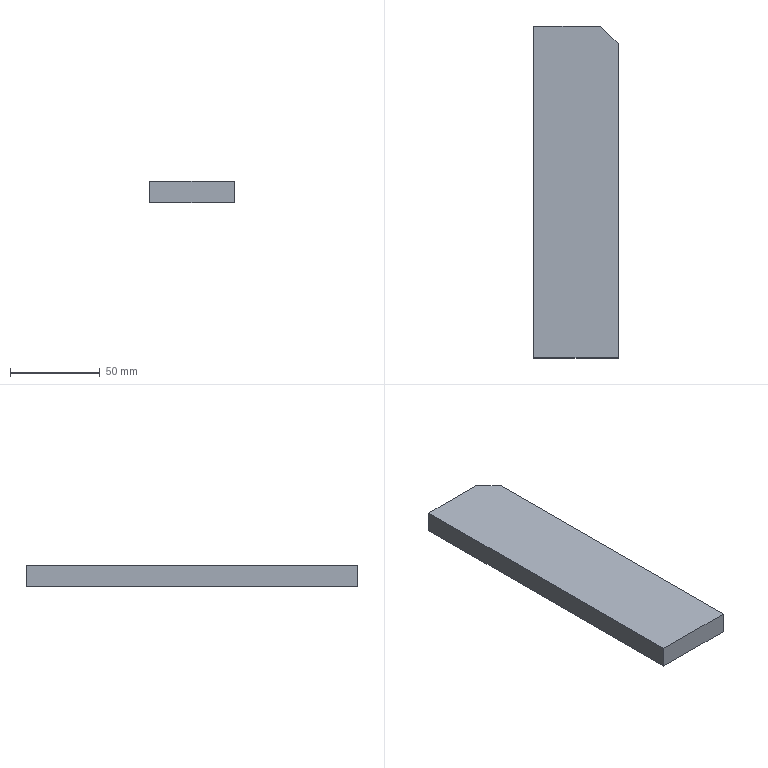Part | SolidWorks | features Chamfer 1, Extrusion 1, Fillet 1, ICE 1 | 1 solid | 7 faces | box 47 x 185 x 12 mm | volume 103740 mm3 | plane 7
STEP:
#1=CARTESIAN_POINT('',(0.,185.,-6.));
#2=VERTEX_POINT('',#1);
#3=CARTESIAN_POINT('',(0.,0.,-6.));
#4=VERTEX_POINT('',#3);
#5=CARTESIAN_POINT('',(0.,185.,-6.));
#6=DIRECTION('',(0.,-1.,0.));
#7=VECTOR('',#6,1000.);
#8=LINE('',#5,#7);
#9=EDGE_CURVE('',#2,#4,#8,.T.);
#10=ORIENTED_EDGE('',*,*,#9,.T.);
#11=CARTESIAN_POINT('',(0.,0.,6.));
#12=VERTEX_POINT('',#11);
#13=CARTESIAN_POINT('',(0.,0.,6.));
#14=DIRECTION('',(0.,0.,-1.));
#15=VECTOR('',#14,1000.);
#16=LINE('',#13,#15);
#17=EDGE_CURVE('',#12,#4,#16,.T.);
#18=ORIENTED_EDGE('',*,*,#17,.F.);
#19=CARTESIAN_POINT('',(0.,185.,6.));
#20=VERTEX_POINT('',#19);
#21=CARTESIAN_POINT('',(0.,185.,6.));
#22=DIRECTION('',(0.,-1.,0.));
#23=VECTOR('',#22,1000.);
#24=LINE('',#21,#23);
#25=EDGE_CURVE('',#20,#12,#24,.T.);
#26=ORIENTED_EDGE('',*,*,#25,.F.);
#27=CARTESIAN_POINT('',(0.,185.,6.));
#28=DIRECTION('',(0.,0.,-1.));
#29=VECTOR('',#28,1000.);
#30=LINE('',#27,#29);
#31=EDGE_CURVE('',#20,#2,#30,.T.);
#32=ORIENTED_EDGE('',*,*,#31,.T.);
#33=EDGE_LOOP('',(#10,#18,#26,#32));
#34=FACE_OUTER_BOUND('',#33,.T.);
#35=CARTESIAN_POINT('',(0.,185.,6.));
#36=DIRECTION('',(1.,0.,0.));
#37=DIRECTION('',(0.,0.,-1.));
#38=AXIS2_PLACEMENT_3D('',#35,#36,#37);
#39=PLANE('',#38);
#40=ADVANCED_FACE('',(#34),#39,.F.);
#41=CARTESIAN_POINT('',(47.,0.,-6.));
#42=VERTEX_POINT('',#41);
#43=CARTESIAN_POINT('',(0.,0.,-6.));
#44=DIRECTION('',(1.,0.,0.));
#45=VECTOR('',#44,1000.);
#46=LINE('',#43,#45);
#47=EDGE_CURVE('',#4,#42,#46,.T.);
#48=ORIENTED_EDGE('',*,*,#47,.T.);
#49=CARTESIAN_POINT('',(47.,0.,6.));
#50=VERTEX_POINT('',#49);
#51=CARTESIAN_POINT('',(47.,0.,6.));
#52=DIRECTION('',(0.,0.,-1.));
#53=VECTOR('',#52,1000.);
#54=LINE('',#51,#53);
#55=EDGE_CURVE('',#50,#42,#54,.T.);
#56=ORIENTED_EDGE('',*,*,#55,.F.);
#57=CARTESIAN_POINT('',(0.,0.,6.));
#58=DIRECTION('',(1.,0.,0.));
#59=VECTOR('',#58,1000.);
#60=LINE('',#57,#59);
#61=EDGE_CURVE('',#12,#50,#60,.T.);
#62=ORIENTED_EDGE('',*,*,#61,.F.);
#63=ORIENTED_EDGE('',*,*,#17,.T.);
#64=EDGE_LOOP('',(#48,#56,#62,#63));
#65=FACE_OUTER_BOUND('',#64,.T.);
#66=CARTESIAN_POINT('',(0.,0.,6.));
#67=DIRECTION('',(0.,1.,0.));
#68=DIRECTION('',(0.,0.,1.));
#69=AXIS2_PLACEMENT_3D('',#66,#67,#68);
#70=PLANE('',#69);
#71=ADVANCED_FACE('',(#65),#70,.F.);
#72=CARTESIAN_POINT('',(47.,175.,-6.));
#73=VERTEX_POINT('',#72);
#74=CARTESIAN_POINT('',(47.,0.,-6.));
#75=DIRECTION('',(0.,1.,0.));
#76=VECTOR('',#75,1000.);
#77=LINE('',#74,#76);
#78=EDGE_CURVE('',#42,#73,#77,.T.);
#79=ORIENTED_EDGE('',*,*,#78,.T.);
#80=CARTESIAN_POINT('',(47.,175.,6.));
#81=VERTEX_POINT('',#80);
#82=CARTESIAN_POINT('',(47.,175.,6.));
#83=DIRECTION('',(0.,0.,1.));
#84=VECTOR('',#83,1000.);
#85=LINE('',#82,#84);
#86=EDGE_CURVE('',#73,#81,#85,.T.);
#87=ORIENTED_EDGE('',*,*,#86,.T.);
#88=CARTESIAN_POINT('',(47.,0.,6.));
#89=DIRECTION('',(0.,1.,0.));
#90=VECTOR('',#89,1000.);
#91=LINE('',#88,#90);
#92=EDGE_CURVE('',#50,#81,#91,.T.);
#93=ORIENTED_EDGE('',*,*,#92,.F.);
#94=ORIENTED_EDGE('',*,*,#55,.T.);
#95=EDGE_LOOP('',(#79,#87,#93,#94));
#96=FACE_OUTER_BOUND('',#95,.T.);
#97=CARTESIAN_POINT('',(47.,0.,6.));
#98=DIRECTION('',(-1.,0.,0.));
#99=DIRECTION('',(0.,0.,1.));
#100=AXIS2_PLACEMENT_3D('',#97,#98,#99);
#101=PLANE('',#100);
#102=ADVANCED_FACE('',(#96),#101,.F.);
#103=CARTESIAN_POINT('',(37.,185.,6.));
#104=VERTEX_POINT('',#103);
#105=CARTESIAN_POINT('',(47.,185.,6.));
#106=DIRECTION('',(-1.,0.,0.));
#107=VECTOR('',#106,1000.);
#108=LINE('',#105,#107);
#109=EDGE_CURVE('',#104,#20,#108,.T.);
#110=ORIENTED_EDGE('',*,*,#109,.F.);
#111=CARTESIAN_POINT('',(37.,185.,-6.));
#112=VERTEX_POINT('',#111);
#113=CARTESIAN_POINT('',(37.,185.,6.));
#114=DIRECTION('',(0.,0.,-1.));
#115=VECTOR('',#114,1000.);
#116=LINE('',#113,#115);
#117=EDGE_CURVE('',#104,#112,#116,.T.);
#118=ORIENTED_EDGE('',*,*,#117,.T.);
#119=CARTESIAN_POINT('',(47.,185.,-6.));
#120=DIRECTION('',(-1.,0.,0.));
#121=VECTOR('',#120,1000.);
#122=LINE('',#119,#121);
#123=EDGE_CURVE('',#112,#2,#122,.T.);
#124=ORIENTED_EDGE('',*,*,#123,.T.);
#125=ORIENTED_EDGE('',*,*,#31,.F.);
#126=EDGE_LOOP('',(#110,#118,#124,#125));
#127=FACE_OUTER_BOUND('',#126,.T.);
#128=CARTESIAN_POINT('',(47.,185.,6.));
#129=DIRECTION('',(0.,-1.,0.));
#130=DIRECTION('',(0.,0.,-1.));
#131=AXIS2_PLACEMENT_3D('',#128,#129,#130);
#132=PLANE('',#131);
#133=ADVANCED_FACE('',(#127),#132,.F.);
#134=ORIENTED_EDGE('',*,*,#92,.T.);
#135=CARTESIAN_POINT('',(111.,111.,6.));
#136=DIRECTION('',(-0.7071,0.7071,0.));
#137=VECTOR('',#136,1000.);
#138=LINE('',#135,#137);
#139=EDGE_CURVE('',#81,#104,#138,.T.);
#140=ORIENTED_EDGE('',*,*,#139,.T.);
#141=ORIENTED_EDGE('',*,*,#109,.T.);
#142=ORIENTED_EDGE('',*,*,#25,.T.);
#143=ORIENTED_EDGE('',*,*,#61,.T.);
#144=EDGE_LOOP('',(#134,#140,#141,#142,#143));
#145=FACE_OUTER_BOUND('',#144,.T.);
#146=CARTESIAN_POINT('',(0.,0.,6.));
#147=DIRECTION('',(0.,0.,1.));
#148=DIRECTION('',(1.,0.,0.));
#149=AXIS2_PLACEMENT_3D('',#146,#147,#148);
#150=PLANE('',#149);
#151=ADVANCED_FACE('',(#145),#150,.T.);
#152=ORIENTED_EDGE('',*,*,#123,.F.);
#153=CARTESIAN_POINT('',(37.,185.,-6.));
#154=DIRECTION('',(0.7071,-0.7071,0.));
#155=VECTOR('',#154,1000.);
#156=LINE('',#153,#155);
#157=EDGE_CURVE('',#112,#73,#156,.T.);
#158=ORIENTED_EDGE('',*,*,#157,.T.);
#159=ORIENTED_EDGE('',*,*,#78,.F.);
#160=ORIENTED_EDGE('',*,*,#47,.F.);
#161=ORIENTED_EDGE('',*,*,#9,.F.);
#162=EDGE_LOOP('',(#152,#158,#159,#160,#161));
#163=FACE_OUTER_BOUND('',#162,.T.);
#164=CARTESIAN_POINT('',(0.,0.,-6.));
#165=DIRECTION('',(0.,0.,1.));
#166=DIRECTION('',(1.,0.,0.));
#167=AXIS2_PLACEMENT_3D('',#164,#165,#166);
#168=PLANE('',#167);
#169=ADVANCED_FACE('',(#163),#168,.F.);
#170=ORIENTED_EDGE('',*,*,#139,.F.);
#171=ORIENTED_EDGE('',*,*,#86,.F.);
#172=ORIENTED_EDGE('',*,*,#157,.F.);
#173=ORIENTED_EDGE('',*,*,#117,.F.);
#174=EDGE_LOOP('',(#170,#171,#172,#173));
#175=FACE_OUTER_BOUND('',#174,.T.);
#176=CARTESIAN_POINT('',(37.,185.,6.));
#177=DIRECTION('',(-0.7071,-0.7071,0.));
#178=DIRECTION('',(0.,0.,-1.));
#179=AXIS2_PLACEMENT_3D('',#176,#177,#178);
#180=PLANE('',#179);
#181=ADVANCED_FACE('',(#175),#180,.F.);
#182=CLOSED_SHELL('',(#40,#71,#102,#133,#151,#169,#181));
#183=MANIFOLD_SOLID_BREP('',#182);
#184=CARTESIAN_POINT('',(0.,0.,0.));
#185=DIRECTION('',(0.,0.,1.));
#186=DIRECTION('',(1.,0.,0.));
#187=AXIS2_PLACEMENT_3D('',#184,#185,#186);
#188=(LENGTH_UNIT()NAMED_UNIT(*)SI_UNIT(.MILLI.,.METRE.));
#189=UNCERTAINTY_MEASURE_WITH_UNIT(LENGTH_MEASURE(0.00001),#188,'','');
#190=(NAMED_UNIT(*)PLANE_ANGLE_UNIT()SI_UNIT($,.RADIAN.));
#191=(NAMED_UNIT(*)SI_UNIT($,.STERADIAN.)SOLID_ANGLE_UNIT());
#192=(GEOMETRIC_REPRESENTATION_CONTEXT(3)GLOBAL_UNCERTAINTY_ASSIGNED_CONTEXT((#189))GLOBAL_UNIT_ASSIGNED_CONTEXT((#188,#190,#191))REPRESENTATION_CONTEXT('',''));
#193=ADVANCED_BREP_SHAPE_REPRESENTATION('',(#183,#187),#192);